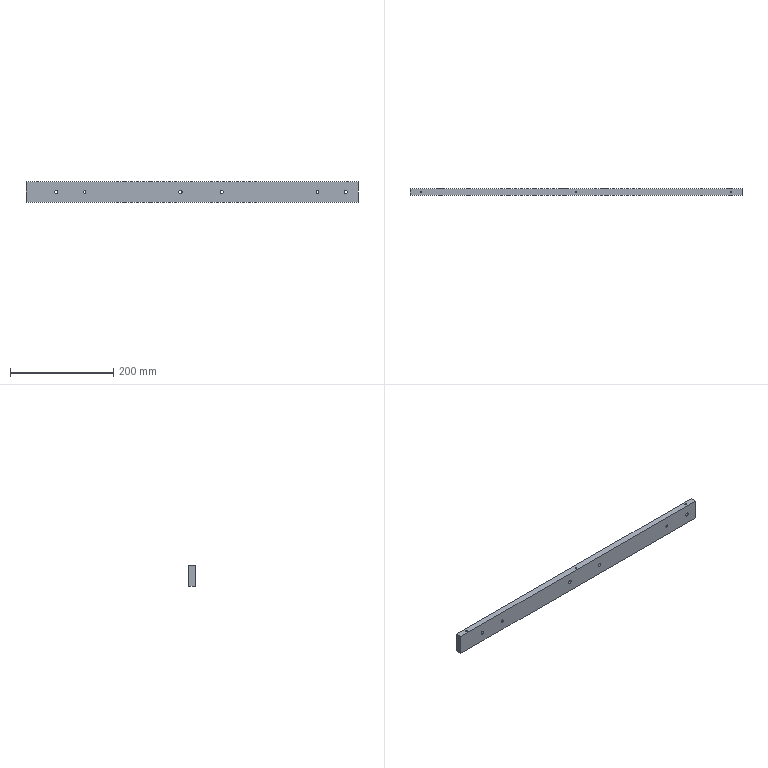Part | SolidWorks | features 3DProfileFeature 3, HoleWzd 3, Extrusion 1 | 1 solid | 42 faces | box 642 x 12 x 40 mm | volume 304076 mm3 | cylinder 26 | plane 10 | cone 6 | commonest cylinder face diameters 6.6 x8 11 x8 3.3 x6 5 x4
STEP:
#1=CARTESIAN_POINT('',(-207.5,-6.,-2.5));
#2=VERTEX_POINT('',#1);
#3=CARTESIAN_POINT('',(-207.5,-6.,2.5));
#4=VERTEX_POINT('',#3);
#5=CARTESIAN_POINT('',(-207.5,-6.,0.));
#6=DIRECTION('',(0.,1.,0.));
#7=DIRECTION('',(0.,0.,1.));
#8=AXIS2_PLACEMENT_3D('',#5,#6,#7);
#9=CIRCLE('',#8,2.5);
#10=EDGE_CURVE('',#2,#4,#9,.T.);
#11=ORIENTED_EDGE('',*,*,#10,.F.);
#12=CARTESIAN_POINT('',(-207.5,6.,-2.5));
#13=VERTEX_POINT('',#12);
#14=CARTESIAN_POINT('',(-207.5,6.,-2.5));
#15=DIRECTION('',(0.,1.,0.));
#16=VECTOR('',#15,1000.);
#17=LINE('',#14,#16);
#18=EDGE_CURVE('',#2,#13,#17,.T.);
#19=ORIENTED_EDGE('',*,*,#18,.T.);
#20=CARTESIAN_POINT('',(-207.5,6.,2.5));
#21=VERTEX_POINT('',#20);
#22=CARTESIAN_POINT('',(-207.5,6.,0.));
#23=DIRECTION('',(0.,1.,0.));
#24=DIRECTION('',(0.,0.,1.));
#25=AXIS2_PLACEMENT_3D('',#22,#23,#24);
#26=CIRCLE('',#25,2.5);
#27=EDGE_CURVE('',#13,#21,#26,.T.);
#28=ORIENTED_EDGE('',*,*,#27,.T.);
#29=CARTESIAN_POINT('',(-207.5,6.,2.5));
#30=DIRECTION('',(0.,1.,0.));
#31=VECTOR('',#30,1000.);
#32=LINE('',#29,#31);
#33=EDGE_CURVE('',#4,#21,#32,.T.);
#34=ORIENTED_EDGE('',*,*,#33,.F.);
#35=EDGE_LOOP('',(#11,#19,#28,#34));
#36=FACE_OUTER_BOUND('',#35,.T.);
#37=CARTESIAN_POINT('',(-207.5,6.,0.));
#38=DIRECTION('',(0.,1.,0.));
#39=DIRECTION('',(0.,0.,1.));
#40=AXIS2_PLACEMENT_3D('',#37,#38,#39);
#41=CYLINDRICAL_SURFACE('',#40,2.5);
#42=ADVANCED_FACE('',(#36),#41,.F.);
#43=CARTESIAN_POINT('',(242.5,-6.,-2.5));
#44=VERTEX_POINT('',#43);
#45=CARTESIAN_POINT('',(242.5,-6.,2.5));
#46=VERTEX_POINT('',#45);
#47=CARTESIAN_POINT('',(242.5,-6.,0.));
#48=DIRECTION('',(0.,1.,0.));
#49=DIRECTION('',(0.,0.,1.));
#50=AXIS2_PLACEMENT_3D('',#47,#48,#49);
#51=CIRCLE('',#50,2.5);
#52=EDGE_CURVE('',#44,#46,#51,.T.);
#53=ORIENTED_EDGE('',*,*,#52,.F.);
#54=CARTESIAN_POINT('',(242.5,6.,-2.5));
#55=VERTEX_POINT('',#54);
#56=CARTESIAN_POINT('',(242.5,6.,-2.5));
#57=DIRECTION('',(0.,1.,0.));
#58=VECTOR('',#57,1000.);
#59=LINE('',#56,#58);
#60=EDGE_CURVE('',#44,#55,#59,.T.);
#61=ORIENTED_EDGE('',*,*,#60,.T.);
#62=CARTESIAN_POINT('',(242.5,6.,2.5));
#63=VERTEX_POINT('',#62);
#64=CARTESIAN_POINT('',(242.5,6.,0.));
#65=DIRECTION('',(0.,1.,0.));
#66=DIRECTION('',(0.,0.,1.));
#67=AXIS2_PLACEMENT_3D('',#64,#65,#66);
#68=CIRCLE('',#67,2.5);
#69=EDGE_CURVE('',#55,#63,#68,.T.);
#70=ORIENTED_EDGE('',*,*,#69,.T.);
#71=CARTESIAN_POINT('',(242.5,6.,2.5));
#72=DIRECTION('',(0.,1.,0.));
#73=VECTOR('',#72,1000.);
#74=LINE('',#71,#73);
#75=EDGE_CURVE('',#46,#63,#74,.T.);
#76=ORIENTED_EDGE('',*,*,#75,.F.);
#77=EDGE_LOOP('',(#53,#61,#70,#76));
#78=FACE_OUTER_BOUND('',#77,.T.);
#79=CARTESIAN_POINT('',(242.5,6.,0.));
#80=DIRECTION('',(0.,1.,0.));
#81=DIRECTION('',(0.,0.,1.));
#82=AXIS2_PLACEMENT_3D('',#79,#80,#81);
#83=CYLINDRICAL_SURFACE('',#82,2.5);
#84=ADVANCED_FACE('',(#78),#83,.F.);
#85=CARTESIAN_POINT('',(300.,0.,8.909));
#86=VERTEX_POINT('',#85);
#87=CARTESIAN_POINT('',(301.65,0.,9.9));
#88=VERTEX_POINT('',#87);
#89=CARTESIAN_POINT('',(301.65,0.,9.9));
#90=DIRECTION('',(0.8572,0.,0.515));
#91=VECTOR('',#90,1000.);
#92=LINE('',#89,#91);
#93=EDGE_CURVE('',#86,#88,#92,.T.);
#94=ORIENTED_EDGE('',*,*,#93,.F.);
#95=CARTESIAN_POINT('',(298.35,0.,9.9));
#96=VERTEX_POINT('',#95);
#97=CARTESIAN_POINT('',(298.35,0.,9.9));
#98=DIRECTION('',(-0.8572,0.,0.515));
#99=VECTOR('',#98,1000.);
#100=LINE('',#97,#99);
#101=EDGE_CURVE('',#86,#96,#100,.T.);
#102=ORIENTED_EDGE('',*,*,#101,.T.);
#103=CARTESIAN_POINT('',(300.,0.,9.9));
#104=DIRECTION('',(0.,0.,1.));
#105=DIRECTION('',(1.,0.,0.));
#106=AXIS2_PLACEMENT_3D('',#103,#104,#105);
#107=CIRCLE('',#106,1.65);
#108=EDGE_CURVE('',#96,#88,#107,.T.);
#109=ORIENTED_EDGE('',*,*,#108,.T.);
#110=EDGE_LOOP('',(#94,#102,#109));
#111=FACE_OUTER_BOUND('',#110,.T.);
#112=CARTESIAN_POINT('',(300.,0.,9.9));
#113=DIRECTION('',(0.,0.,1.));
#114=DIRECTION('',(1.,0.,0.));
#115=AXIS2_PLACEMENT_3D('',#112,#113,#114);
#116=CONICAL_SURFACE('',#115,1.65,1.03);
#117=ADVANCED_FACE('',(#111),#116,.F.);
#118=ORIENTED_EDGE('',*,*,#108,.F.);
#119=CARTESIAN_POINT('',(298.35,0.,20.));
#120=VERTEX_POINT('',#119);
#121=CARTESIAN_POINT('',(298.35,0.,20.));
#122=DIRECTION('',(0.,0.,1.));
#123=VECTOR('',#122,1000.);
#124=LINE('',#121,#123);
#125=EDGE_CURVE('',#96,#120,#124,.T.);
#126=ORIENTED_EDGE('',*,*,#125,.T.);
#127=CARTESIAN_POINT('',(301.65,0.,20.));
#128=VERTEX_POINT('',#127);
#129=CARTESIAN_POINT('',(300.,0.,20.));
#130=DIRECTION('',(0.,0.,1.));
#131=DIRECTION('',(1.,0.,0.));
#132=AXIS2_PLACEMENT_3D('',#129,#130,#131);
#133=CIRCLE('',#132,1.65);
#134=EDGE_CURVE('',#120,#128,#133,.T.);
#135=ORIENTED_EDGE('',*,*,#134,.T.);
#136=CARTESIAN_POINT('',(301.65,0.,20.));
#137=DIRECTION('',(0.,0.,1.));
#138=VECTOR('',#137,1000.);
#139=LINE('',#136,#138);
#140=EDGE_CURVE('',#88,#128,#139,.T.);
#141=ORIENTED_EDGE('',*,*,#140,.F.);
#142=EDGE_LOOP('',(#118,#126,#135,#141));
#143=FACE_OUTER_BOUND('',#142,.T.);
#144=CARTESIAN_POINT('',(300.,0.,20.));
#145=DIRECTION('',(0.,0.,1.));
#146=DIRECTION('',(1.,0.,0.));
#147=AXIS2_PLACEMENT_3D('',#144,#145,#146);
#148=CYLINDRICAL_SURFACE('',#147,1.65);
#149=ADVANCED_FACE('',(#143),#148,.F.);
#150=CARTESIAN_POINT('',(0.,0.,8.909));
#151=VERTEX_POINT('',#150);
#152=CARTESIAN_POINT('',(1.65,0.,9.9));
#153=VERTEX_POINT('',#152);
#154=CARTESIAN_POINT('',(1.65,0.,9.9));
#155=DIRECTION('',(0.8572,0.,0.515));
#156=VECTOR('',#155,1000.);
#157=LINE('',#154,#156);
#158=EDGE_CURVE('',#151,#153,#157,.T.);
#159=ORIENTED_EDGE('',*,*,#158,.F.);
#160=CARTESIAN_POINT('',(-1.65,0.,9.9));
#161=VERTEX_POINT('',#160);
#162=CARTESIAN_POINT('',(-1.65,0.,9.9));
#163=DIRECTION('',(-0.8572,0.,0.515));
#164=VECTOR('',#163,1000.);
#165=LINE('',#162,#164);
#166=EDGE_CURVE('',#151,#161,#165,.T.);
#167=ORIENTED_EDGE('',*,*,#166,.T.);
#168=CARTESIAN_POINT('',(0.,0.,9.9));
#169=DIRECTION('',(0.,0.,1.));
#170=DIRECTION('',(1.,0.,0.));
#171=AXIS2_PLACEMENT_3D('',#168,#169,#170);
#172=CIRCLE('',#171,1.65);
#173=EDGE_CURVE('',#161,#153,#172,.T.);
#174=ORIENTED_EDGE('',*,*,#173,.T.);
#175=EDGE_LOOP('',(#159,#167,#174));
#176=FACE_OUTER_BOUND('',#175,.T.);
#177=CARTESIAN_POINT('',(0.,0.,9.9));
#178=DIRECTION('',(0.,0.,1.));
#179=DIRECTION('',(1.,0.,0.));
#180=AXIS2_PLACEMENT_3D('',#177,#178,#179);
#181=CONICAL_SURFACE('',#180,1.65,1.03);
#182=ADVANCED_FACE('',(#176),#181,.F.);
#183=ORIENTED_EDGE('',*,*,#173,.F.);
#184=CARTESIAN_POINT('',(-1.65,0.,20.));
#185=VERTEX_POINT('',#184);
#186=CARTESIAN_POINT('',(-1.65,0.,20.));
#187=DIRECTION('',(0.,0.,1.));
#188=VECTOR('',#187,1000.);
#189=LINE('',#186,#188);
#190=EDGE_CURVE('',#161,#185,#189,.T.);
#191=ORIENTED_EDGE('',*,*,#190,.T.);
#192=CARTESIAN_POINT('',(1.65,0.,20.));
#193=VERTEX_POINT('',#192);
#194=CARTESIAN_POINT('',(0.,0.,20.));
#195=DIRECTION('',(0.,0.,1.));
#196=DIRECTION('',(1.,0.,0.));
#197=AXIS2_PLACEMENT_3D('',#194,#195,#196);
#198=CIRCLE('',#197,1.65);
#199=EDGE_CURVE('',#185,#193,#198,.T.);
#200=ORIENTED_EDGE('',*,*,#199,.T.);
#201=CARTESIAN_POINT('',(1.65,0.,20.));
#202=DIRECTION('',(0.,0.,1.));
#203=VECTOR('',#202,1000.);
#204=LINE('',#201,#203);
#205=EDGE_CURVE('',#153,#193,#204,.T.);
#206=ORIENTED_EDGE('',*,*,#205,.F.);
#207=EDGE_LOOP('',(#183,#191,#200,#206));
#208=FACE_OUTER_BOUND('',#207,.T.);
#209=CARTESIAN_POINT('',(0.,0.,20.));
#210=DIRECTION('',(0.,0.,1.));
#211=DIRECTION('',(1.,0.,0.));
#212=AXIS2_PLACEMENT_3D('',#209,#210,#211);
#213=CYLINDRICAL_SURFACE('',#212,1.65);
#214=ADVANCED_FACE('',(#208),#213,.F.);
#215=CARTESIAN_POINT('',(-300.,0.,8.909));
#216=VERTEX_POINT('',#215);
#217=CARTESIAN_POINT('',(-298.35,0.,9.9));
#218=VERTEX_POINT('',#217);
#219=CARTESIAN_POINT('',(-298.35,0.,9.9));
#220=DIRECTION('',(0.8572,0.,0.515));
#221=VECTOR('',#220,1000.);
#222=LINE('',#219,#221);
#223=EDGE_CURVE('',#216,#218,#222,.T.);
#224=ORIENTED_EDGE('',*,*,#223,.F.);
#225=CARTESIAN_POINT('',(-301.65,0.,9.9));
#226=VERTEX_POINT('',#225);
#227=CARTESIAN_POINT('',(-301.65,0.,9.9));
#228=DIRECTION('',(-0.8572,0.,0.515));
#229=VECTOR('',#228,1000.);
#230=LINE('',#227,#229);
#231=EDGE_CURVE('',#216,#226,#230,.T.);
#232=ORIENTED_EDGE('',*,*,#231,.T.);
#233=CARTESIAN_POINT('',(-300.,0.,9.9));
#234=DIRECTION('',(0.,0.,1.));
#235=DIRECTION('',(1.,0.,0.));
#236=AXIS2_PLACEMENT_3D('',#233,#234,#235);
#237=CIRCLE('',#236,1.65);
#238=EDGE_CURVE('',#226,#218,#237,.T.);
#239=ORIENTED_EDGE('',*,*,#238,.T.);
#240=EDGE_LOOP('',(#224,#232,#239));
#241=FACE_OUTER_BOUND('',#240,.T.);
#242=CARTESIAN_POINT('',(-300.,0.,9.9));
#243=DIRECTION('',(0.,0.,1.));
#244=DIRECTION('',(1.,0.,0.));
#245=AXIS2_PLACEMENT_3D('',#242,#243,#244);
#246=CONICAL_SURFACE('',#245,1.65,1.03);
#247=ADVANCED_FACE('',(#241),#246,.F.);
#248=ORIENTED_EDGE('',*,*,#238,.F.);
#249=CARTESIAN_POINT('',(-301.65,0.,20.));
#250=VERTEX_POINT('',#249);
#251=CARTESIAN_POINT('',(-301.65,0.,20.));
#252=DIRECTION('',(0.,0.,1.));
#253=VECTOR('',#252,1000.);
#254=LINE('',#251,#253);
#255=EDGE_CURVE('',#226,#250,#254,.T.);
#256=ORIENTED_EDGE('',*,*,#255,.T.);
#257=CARTESIAN_POINT('',(-298.35,0.,20.));
#258=VERTEX_POINT('',#257);
#259=CARTESIAN_POINT('',(-300.,0.,20.));
#260=DIRECTION('',(0.,0.,1.));
#261=DIRECTION('',(1.,0.,0.));
#262=AXIS2_PLACEMENT_3D('',#259,#260,#261);
#263=CIRCLE('',#262,1.65);
#264=EDGE_CURVE('',#250,#258,#263,.T.);
#265=ORIENTED_EDGE('',*,*,#264,.T.);
#266=CARTESIAN_POINT('',(-298.35,0.,20.));
#267=DIRECTION('',(0.,0.,1.));
#268=VECTOR('',#267,1000.);
#269=LINE('',#266,#268);
#270=EDGE_CURVE('',#218,#258,#269,.T.);
#271=ORIENTED_EDGE('',*,*,#270,.F.);
#272=EDGE_LOOP('',(#248,#256,#265,#271));
#273=FACE_OUTER_BOUND('',#272,.T.);
#274=CARTESIAN_POINT('',(-300.,0.,20.));
#275=DIRECTION('',(0.,0.,1.));
#276=DIRECTION('',(1.,0.,0.));
#277=AXIS2_PLACEMENT_3D('',#274,#275,#276);
#278=CYLINDRICAL_SURFACE('',#277,1.65);
#279=ADVANCED_FACE('',(#273),#278,.F.);
#280=CARTESIAN_POINT('',(-262.5,-1.,-5.5));
#281=VERTEX_POINT('',#280);
#282=CARTESIAN_POINT('',(-262.5,-1.,5.5));
#283=VERTEX_POINT('',#282);
#284=CARTESIAN_POINT('',(-262.5,-1.,0.));
#285=DIRECTION('',(0.,1.,0.));
#286=DIRECTION('',(0.,0.,1.));
#287=AXIS2_PLACEMENT_3D('',#284,#285,#286);
#288=CIRCLE('',#287,5.5);
#289=EDGE_CURVE('',#281,#283,#288,.T.);
#290=ORIENTED_EDGE('',*,*,#289,.F.);
#291=CARTESIAN_POINT('',(-262.5,6.,-5.5));
#292=VERTEX_POINT('',#291);
#293=CARTESIAN_POINT('',(-262.5,6.,-5.5));
#294=DIRECTION('',(0.,1.,0.));
#295=VECTOR('',#294,1000.);
#296=LINE('',#293,#295);
#297=EDGE_CURVE('',#281,#292,#296,.T.);
#298=ORIENTED_EDGE('',*,*,#297,.T.);
#299=CARTESIAN_POINT('',(-262.5,6.,5.5));
#300=VERTEX_POINT('',#299);
#301=CARTESIAN_POINT('',(-262.5,6.,0.));
#302=DIRECTION('',(0.,1.,0.));
#303=DIRECTION('',(0.,0.,1.));
#304=AXIS2_PLACEMENT_3D('',#301,#302,#303);
#305=CIRCLE('',#304,5.5);
#306=EDGE_CURVE('',#292,#300,#305,.T.);
#307=ORIENTED_EDGE('',*,*,#306,.T.);
#308=CARTESIAN_POINT('',(-262.5,6.,5.5));
#309=DIRECTION('',(0.,1.,0.));
#310=VECTOR('',#309,1000.);
#311=LINE('',#308,#310);
#312=EDGE_CURVE('',#283,#300,#311,.T.);
#313=ORIENTED_EDGE('',*,*,#312,.F.);
#314=EDGE_LOOP('',(#290,#298,#307,#313));
#315=FACE_OUTER_BOUND('',#314,.T.);
#316=CARTESIAN_POINT('',(-262.5,6.,0.));
#317=DIRECTION('',(0.,1.,0.));
#318=DIRECTION('',(0.,0.,1.));
#319=AXIS2_PLACEMENT_3D('',#316,#317,#318);
#320=CYLINDRICAL_SURFACE('',#319,5.5);
#321=ADVANCED_FACE('',(#315),#320,.F.);
#322=CARTESIAN_POINT('',(-262.5,-6.,-3.3));
#323=VERTEX_POINT('',#322);
#324=CARTESIAN_POINT('',(-262.5,-6.,3.3));
#325=VERTEX_POINT('',#324);
#326=CARTESIAN_POINT('',(-262.5,-6.,0.));
#327=DIRECTION('',(0.,1.,0.));
#328=DIRECTION('',(0.,0.,1.));
#329=AXIS2_PLACEMENT_3D('',#326,#327,#328);
#330=CIRCLE('',#329,3.3);
#331=EDGE_CURVE('',#323,#325,#330,.T.);
#332=ORIENTED_EDGE('',*,*,#331,.F.);
#333=CARTESIAN_POINT('',(-262.5,-1.,-3.3));
#334=VERTEX_POINT('',#333);
#335=CARTESIAN_POINT('',(-262.5,6.,-3.3));
#336=DIRECTION('',(0.,1.,0.));
#337=VECTOR('',#336,1000.);
#338=LINE('',#335,#337);
#339=EDGE_CURVE('',#323,#334,#338,.T.);
#340=ORIENTED_EDGE('',*,*,#339,.T.);
#341=CARTESIAN_POINT('',(-262.5,-1.,3.3));
#342=VERTEX_POINT('',#341);
#343=CARTESIAN_POINT('',(-262.5,-1.,0.));
#344=DIRECTION('',(0.,1.,0.));
#345=DIRECTION('',(0.,0.,1.));
#346=AXIS2_PLACEMENT_3D('',#343,#344,#345);
#347=CIRCLE('',#346,3.3);
#348=EDGE_CURVE('',#334,#342,#347,.T.);
#349=ORIENTED_EDGE('',*,*,#348,.T.);
#350=CARTESIAN_POINT('',(-262.5,6.,3.3));
#351=DIRECTION('',(0.,1.,0.));
#352=VECTOR('',#351,1000.);
#353=LINE('',#350,#352);
#354=EDGE_CURVE('',#325,#342,#353,.T.);
#355=ORIENTED_EDGE('',*,*,#354,.F.);
#356=EDGE_LOOP('',(#332,#340,#349,#355));
#357=FACE_OUTER_BOUND('',#356,.T.);
#358=CARTESIAN_POINT('',(-262.5,6.,0.));
#359=DIRECTION('',(0.,1.,0.));
#360=DIRECTION('',(0.,0.,1.));
#361=AXIS2_PLACEMENT_3D('',#358,#359,#360);
#362=CYLINDRICAL_SURFACE('',#361,3.3);
#363=ADVANCED_FACE('',(#357),#362,.F.);
#364=CARTESIAN_POINT('',(-22.5,-1.,-5.5));
#365=VERTEX_POINT('',#364);
#366=CARTESIAN_POINT('',(-22.5,-1.,5.5));
#367=VERTEX_POINT('',#366);
#368=CARTESIAN_POINT('',(-22.5,-1.,0.));
#369=DIRECTION('',(0.,1.,0.));
#370=DIRECTION('',(0.,0.,1.));
#371=AXIS2_PLACEMENT_3D('',#368,#369,#370);
#372=CIRCLE('',#371,5.5);
#373=EDGE_CURVE('',#365,#367,#372,.T.);
#374=ORIENTED_EDGE('',*,*,#373,.F.);
#375=CARTESIAN_POINT('',(-22.5,6.,-5.5));
#376=VERTEX_POINT('',#375);
#377=CARTESIAN_POINT('',(-22.5,6.,-5.5));
#378=DIRECTION('',(0.,1.,0.));
#379=VECTOR('',#378,1000.);
#380=LINE('',#377,#379);
#381=EDGE_CURVE('',#365,#376,#380,.T.);
#382=ORIENTED_EDGE('',*,*,#381,.T.);
#383=CARTESIAN_POINT('',(-22.5,6.,5.5));
#384=VERTEX_POINT('',#383);
#385=CARTESIAN_POINT('',(-22.5,6.,0.));
#386=DIRECTION('',(0.,1.,0.));
#387=DIRECTION('',(0.,0.,1.));
#388=AXIS2_PLACEMENT_3D('',#385,#386,#387);
#389=CIRCLE('',#388,5.5);
#390=EDGE_CURVE('',#376,#384,#389,.T.);
#391=ORIENTED_EDGE('',*,*,#390,.T.);
#392=CARTESIAN_POINT('',(-22.5,6.,5.5));
#393=DIRECTION('',(0.,1.,0.));
#394=VECTOR('',#393,1000.);
#395=LINE('',#392,#394);
#396=EDGE_CURVE('',#367,#384,#395,.T.);
#397=ORIENTED_EDGE('',*,*,#396,.F.);
#398=EDGE_LOOP('',(#374,#382,#391,#397));
#399=FACE_OUTER_BOUND('',#398,.T.);
#400=CARTESIAN_POINT('',(-22.5,6.,0.));
#401=DIRECTION('',(0.,1.,0.));
#402=DIRECTION('',(0.,0.,1.));
#403=AXIS2_PLACEMENT_3D('',#400,#401,#402);
#404=CYLINDRICAL_SURFACE('',#403,5.5);
#405=ADVANCED_FACE('',(#399),#404,.F.);
#406=CARTESIAN_POINT('',(-22.5,-6.,-3.3));
#407=VERTEX_POINT('',#406);
#408=CARTESIAN_POINT('',(-22.5,-6.,3.3));
#409=VERTEX_POINT('',#408);
#410=CARTESIAN_POINT('',(-22.5,-6.,0.));
#411=DIRECTION('',(0.,1.,0.));
#412=DIRECTION('',(0.,0.,1.));
#413=AXIS2_PLACEMENT_3D('',#410,#411,#412);
#414=CIRCLE('',#413,3.3);
#415=EDGE_CURVE('',#407,#409,#414,.T.);
#416=ORIENTED_EDGE('',*,*,#415,.F.);
#417=CARTESIAN_POINT('',(-22.5,-1.,-3.3));
#418=VERTEX_POINT('',#417);
#419=CARTESIAN_POINT('',(-22.5,6.,-3.3));
#420=DIRECTION('',(0.,1.,0.));
#421=VECTOR('',#420,1000.);
#422=LINE('',#419,#421);
#423=EDGE_CURVE('',#407,#418,#422,.T.);
#424=ORIENTED_EDGE('',*,*,#423,.T.);
#425=CARTESIAN_POINT('',(-22.5,-1.,3.3));
#426=VERTEX_POINT('',#425);
#427=CARTESIAN_POINT('',(-22.5,-1.,0.));
#428=DIRECTION('',(0.,1.,0.));
#429=DIRECTION('',(0.,0.,1.));
#430=AXIS2_PLACEMENT_3D('',#427,#428,#429);
#431=CIRCLE('',#430,3.3);
#432=EDGE_CURVE('',#418,#426,#431,.T.);
#433=ORIENTED_EDGE('',*,*,#432,.T.);
#434=CARTESIAN_POINT('',(-22.5,6.,3.3));
#435=DIRECTION('',(0.,1.,0.));
#436=VECTOR('',#435,1000.);
#437=LINE('',#434,#436);
#438=EDGE_CURVE('',#409,#426,#437,.T.);
#439=ORIENTED_EDGE('',*,*,#438,.F.);
#440=EDGE_LOOP('',(#416,#424,#433,#439));
#441=FACE_OUTER_BOUND('',#440,.T.);
#442=CARTESIAN_POINT('',(-22.5,6.,0.));
#443=DIRECTION('',(0.,1.,0.));
#444=DIRECTION('',(0.,0.,1.));
#445=AXIS2_PLACEMENT_3D('',#442,#443,#444);
#446=CYLINDRICAL_SURFACE('',#445,3.3);
#447=ADVANCED_FACE('',(#441),#446,.F.);
#448=CARTESIAN_POINT('',(57.5,-1.,-5.5));
#449=VERTEX_POINT('',#448);
#450=CARTESIAN_POINT('',(57.5,-1.,5.5));
#451=VERTEX_POINT('',#450);
#452=CARTESIAN_POINT('',(57.5,-1.,0.));
#453=DIRECTION('',(0.,1.,0.));
#454=DIRECTION('',(0.,0.,1.));
#455=AXIS2_PLACEMENT_3D('',#452,#453,#454);
#456=CIRCLE('',#455,5.5);
#457=EDGE_CURVE('',#449,#451,#456,.T.);
#458=ORIENTED_EDGE('',*,*,#457,.F.);
#459=CARTESIAN_POINT('',(57.5,6.,-5.5));
#460=VERTEX_POINT('',#459);
#461=CARTESIAN_POINT('',(57.5,6.,-5.5));
#462=DIRECTION('',(0.,1.,0.));
#463=VECTOR('',#462,1000.);
#464=LINE('',#461,#463);
#465=EDGE_CURVE('',#449,#460,#464,.T.);
#466=ORIENTED_EDGE('',*,*,#465,.T.);
#467=CARTESIAN_POINT('',(57.5,6.,5.5));
#468=VERTEX_POINT('',#467);
#469=CARTESIAN_POINT('',(57.5,6.,0.));
#470=DIRECTION('',(0.,1.,0.));
#471=DIRECTION('',(0.,0.,1.));
#472=AXIS2_PLACEMENT_3D('',#469,#470,#471);
#473=CIRCLE('',#472,5.5);
#474=EDGE_CURVE('',#460,#468,#473,.T.);
#475=ORIENTED_EDGE('',*,*,#474,.T.);
#476=CARTESIAN_POINT('',(57.5,6.,5.5));
#477=DIRECTION('',(0.,1.,0.));
#478=VECTOR('',#477,1000.);
#479=LINE('',#476,#478);
#480=EDGE_CURVE('',#451,#468,#479,.T.);
#481=ORIENTED_EDGE('',*,*,#480,.F.);
#482=EDGE_LOOP('',(#458,#466,#475,#481));
#483=FACE_OUTER_BOUND('',#482,.T.);
#484=CARTESIAN_POINT('',(57.5,6.,0.));
#485=DIRECTION('',(0.,1.,0.));
#486=DIRECTION('',(0.,0.,1.));
#487=AXIS2_PLACEMENT_3D('',#484,#485,#486);
#488=CYLINDRICAL_SURFACE('',#487,5.5);
#489=ADVANCED_FACE('',(#483),#488,.F.);
#490=CARTESIAN_POINT('',(57.5,-6.,-3.3));
#491=VERTEX_POINT('',#490);
#492=CARTESIAN_POINT('',(57.5,-6.,3.3));
#493=VERTEX_POINT('',#492);
#494=CARTESIAN_POINT('',(57.5,-6.,0.));
#495=DIRECTION('',(0.,1.,0.));
#496=DIRECTION('',(0.,0.,1.));
#497=AXIS2_PLACEMENT_3D('',#494,#495,#496);
#498=CIRCLE('',#497,3.3);
#499=EDGE_CURVE('',#491,#493,#498,.T.);
#500=ORIENTED_EDGE('',*,*,#499,.F.);
#501=CARTESIAN_POINT('',(57.5,-1.,-3.3));
#502=VERTEX_POINT('',#501);
#503=CARTESIAN_POINT('',(57.5,6.,-3.3));
#504=DIRECTION('',(0.,1.,0.));
#505=VECTOR('',#504,1000.);
#506=LINE('',#503,#505);
#507=EDGE_CURVE('',#491,#502,#506,.T.);
#508=ORIENTED_EDGE('',*,*,#507,.T.);
#509=CARTESIAN_POINT('',(57.5,-1.,3.3));
#510=VERTEX_POINT('',#509);
#511=CARTESIAN_POINT('',(57.5,-1.,0.));
#512=DIRECTION('',(0.,1.,0.));
#513=DIRECTION('',(0.,0.,1.));
#514=AXIS2_PLACEMENT_3D('',#511,#512,#513);
#515=CIRCLE('',#514,3.3);
#516=EDGE_CURVE('',#502,#510,#515,.T.);
#517=ORIENTED_EDGE('',*,*,#516,.T.);
#518=CARTESIAN_POINT('',(57.5,6.,3.3));
#519=DIRECTION('',(0.,1.,0.));
#520=VECTOR('',#519,1000.);
#521=LINE('',#518,#520);
#522=EDGE_CURVE('',#493,#510,#521,.T.);
#523=ORIENTED_EDGE('',*,*,#522,.F.);
#524=EDGE_LOOP('',(#500,#508,#517,#523));
#525=FACE_OUTER_BOUND('',#524,.T.);
#526=CARTESIAN_POINT('',(57.5,6.,0.));
#527=DIRECTION('',(0.,1.,0.));
#528=DIRECTION('',(0.,0.,1.));
#529=AXIS2_PLACEMENT_3D('',#526,#527,#528);
#530=CYLINDRICAL_SURFACE('',#529,3.3);
#531=ADVANCED_FACE('',(#525),#530,.F.);
#532=CARTESIAN_POINT('',(297.5,-1.,-5.5));
#533=VERTEX_POINT('',#532);
#534=CARTESIAN_POINT('',(297.5,-1.,5.5));
#535=VERTEX_POINT('',#534);
#536=CARTESIAN_POINT('',(297.5,-1.,0.));
#537=DIRECTION('',(0.,1.,0.));
#538=DIRECTION('',(0.,0.,1.));
#539=AXIS2_PLACEMENT_3D('',#536,#537,#538);
#540=CIRCLE('',#539,5.5);
#541=EDGE_CURVE('',#533,#535,#540,.T.);
#542=ORIENTED_EDGE('',*,*,#541,.F.);
#543=CARTESIAN_POINT('',(297.5,6.,-5.5));
#544=VERTEX_POINT('',#543);
#545=CARTESIAN_POINT('',(297.5,6.,-5.5));
#546=DIRECTION('',(0.,1.,0.));
#547=VECTOR('',#546,1000.);
#548=LINE('',#545,#547);
#549=EDGE_CURVE('',#533,#544,#548,.T.);
#550=ORIENTED_EDGE('',*,*,#549,.T.);
#551=CARTESIAN_POINT('',(297.5,6.,5.5));
#552=VERTEX_POINT('',#551);
#553=CARTESIAN_POINT('',(297.5,6.,0.));
#554=DIRECTION('',(0.,1.,0.));
#555=DIRECTION('',(0.,0.,1.));
#556=AXIS2_PLACEMENT_3D('',#553,#554,#555);
#557=CIRCLE('',#556,5.5);
#558=EDGE_CURVE('',#544,#552,#557,.T.);
#559=ORIENTED_EDGE('',*,*,#558,.T.);
#560=CARTESIAN_POINT('',(297.5,6.,5.5));
#561=DIRECTION('',(0.,1.,0.));
#562=VECTOR('',#561,1000.);
#563=LINE('',#560,#562);
#564=EDGE_CURVE('',#535,#552,#563,.T.);
#565=ORIENTED_EDGE('',*,*,#564,.F.);
#566=EDGE_LOOP('',(#542,#550,#559,#565));
#567=FACE_OUTER_BOUND('',#566,.T.);
#568=CARTESIAN_POINT('',(297.5,6.,0.));
#569=DIRECTION('',(0.,1.,0.));
#570=DIRECTION('',(0.,0.,1.));
#571=AXIS2_PLACEMENT_3D('',#568,#569,#570);
#572=CYLINDRICAL_SURFACE('',#571,5.5);
#573=ADVANCED_FACE('',(#567),#572,.F.);
#574=CARTESIAN_POINT('',(297.5,-6.,-3.3));
#575=VERTEX_POINT('',#574);
#576=CARTESIAN_POINT('',(297.5,-6.,3.3));
#577=VERTEX_POINT('',#576);
#578=CARTESIAN_POINT('',(297.5,-6.,0.));
#579=DIRECTION('',(0.,1.,0.));
#580=DIRECTION('',(0.,0.,1.));
#581=AXIS2_PLACEMENT_3D('',#578,#579,#580);
#582=CIRCLE('',#581,3.3);
#583=EDGE_CURVE('',#575,#577,#582,.T.);
#584=ORIENTED_EDGE('',*,*,#583,.F.);
#585=CARTESIAN_POINT('',(297.5,-1.,-3.3));
#586=VERTEX_POINT('',#585);
#587=CARTESIAN_POINT('',(297.5,6.,-3.3));
#588=DIRECTION('',(0.,1.,0.));
#589=VECTOR('',#588,1000.);
#590=LINE('',#587,#589);
#591=EDGE_CURVE('',#575,#586,#590,.T.);
#592=ORIENTED_EDGE('',*,*,#591,.T.);
#593=CARTESIAN_POINT('',(297.5,-1.,3.3));
#594=VERTEX_POINT('',#593);
#595=CARTESIAN_POINT('',(297.5,-1.,0.));
#596=DIRECTION('',(0.,1.,0.));
#597=DIRECTION('',(0.,0.,1.));
#598=AXIS2_PLACEMENT_3D('',#595,#596,#597);
#599=CIRCLE('',#598,3.3);
#600=EDGE_CURVE('',#586,#594,#599,.T.);
#601=ORIENTED_EDGE('',*,*,#600,.T.);
#602=CARTESIAN_POINT('',(297.5,6.,3.3));
#603=DIRECTION('',(0.,1.,0.));
#604=VECTOR('',#603,1000.);
#605=LINE('',#602,#604);
#606=EDGE_CURVE('',#577,#594,#605,.T.);
#607=ORIENTED_EDGE('',*,*,#606,.F.);
#608=EDGE_LOOP('',(#584,#592,#601,#607));
#609=FACE_OUTER_BOUND('',#608,.T.);
#610=CARTESIAN_POINT('',(297.5,6.,0.));
#611=DIRECTION('',(0.,1.,0.));
#612=DIRECTION('',(0.,0.,1.));
#613=AXIS2_PLACEMENT_3D('',#610,#611,#612);
#614=CYLINDRICAL_SURFACE('',#613,3.3);
#615=ADVANCED_FACE('',(#609),#614,.F.);
#616=CARTESIAN_POINT('',(-321.,-6.,-20.));
#617=VERTEX_POINT('',#616);
#618=CARTESIAN_POINT('',(-321.,-6.,20.));
#619=VERTEX_POINT('',#618);
#620=CARTESIAN_POINT('',(-321.,-6.,-20.));
#621=DIRECTION('',(0.,0.,1.));
#622=VECTOR('',#621,1000.);
#623=LINE('',#620,#622);
#624=EDGE_CURVE('',#617,#619,#623,.T.);
#625=ORIENTED_EDGE('',*,*,#624,.T.);
#626=CARTESIAN_POINT('',(-321.,6.,20.));
#627=VERTEX_POINT('',#626);
#628=CARTESIAN_POINT('',(-321.,6.,20.));
#629=DIRECTION('',(0.,-1.,0.));
#630=VECTOR('',#629,1000.);
#631=LINE('',#628,#630);
#632=EDGE_CURVE('',#627,#619,#631,.T.);
#633=ORIENTED_EDGE('',*,*,#632,.F.);
#634=CARTESIAN_POINT('',(-321.,6.,-20.));
#635=VERTEX_POINT('',#634);
#636=CARTESIAN_POINT('',(-321.,6.,-20.));
#637=DIRECTION('',(0.,0.,1.));
#638=VECTOR('',#637,1000.);
#639=LINE('',#636,#638);
#640=EDGE_CURVE('',#635,#627,#639,.T.);
#641=ORIENTED_EDGE('',*,*,#640,.F.);
#642=CARTESIAN_POINT('',(-321.,6.,-20.));
#643=DIRECTION('',(0.,-1.,0.));
#644=VECTOR('',#643,1000.);
#645=LINE('',#642,#644);
#646=EDGE_CURVE('',#635,#617,#645,.T.);
#647=ORIENTED_EDGE('',*,*,#646,.T.);
#648=EDGE_LOOP('',(#625,#633,#641,#647));
#649=FACE_OUTER_BOUND('',#648,.T.);
#650=CARTESIAN_POINT('',(-321.,6.,-20.));
#651=DIRECTION('',(1.,0.,0.));
#652=DIRECTION('',(0.,0.,-1.));
#653=AXIS2_PLACEMENT_3D('',#650,#651,#652);
#654=PLANE('',#653);
#655=ADVANCED_FACE('',(#649),#654,.F.);
#656=CARTESIAN_POINT('',(300.,0.,20.));
#657=DIRECTION('',(0.,0.,1.));
#658=DIRECTION('',(1.,0.,0.));
#659=AXIS2_PLACEMENT_3D('',#656,#657,#658);
#660=CIRCLE('',#659,1.65);
#661=EDGE_CURVE('',#128,#120,#660,.T.);
#662=ORIENTED_EDGE('',*,*,#661,.F.);
#663=ORIENTED_EDGE('',*,*,#134,.F.);
#664=EDGE_LOOP('',(#662,#663));
#665=FACE_BOUND('',#664,.T.);
#666=CARTESIAN_POINT('',(0.,0.,20.));
#667=DIRECTION('',(0.,0.,1.));
#668=DIRECTION('',(1.,0.,0.));
#669=AXIS2_PLACEMENT_3D('',#666,#667,#668);
#670=CIRCLE('',#669,1.65);
#671=EDGE_CURVE('',#193,#185,#670,.T.);
#672=ORIENTED_EDGE('',*,*,#671,.F.);
#673=ORIENTED_EDGE('',*,*,#199,.F.);
#674=EDGE_LOOP('',(#672,#673));
#675=FACE_BOUND('',#674,.T.);
#676=CARTESIAN_POINT('',(-300.,0.,20.));
#677=DIRECTION('',(0.,0.,1.));
#678=DIRECTION('',(1.,0.,0.));
#679=AXIS2_PLACEMENT_3D('',#676,#677,#678);
#680=CIRCLE('',#679,1.65);
#681=EDGE_CURVE('',#258,#250,#680,.T.);
#682=ORIENTED_EDGE('',*,*,#681,.F.);
#683=ORIENTED_EDGE('',*,*,#264,.F.);
#684=EDGE_LOOP('',(#682,#683));
#685=FACE_BOUND('',#684,.T.);
#686=CARTESIAN_POINT('',(321.,-6.,20.));
#687=VERTEX_POINT('',#686);
#688=CARTESIAN_POINT('',(-321.,-6.,20.));
#689=DIRECTION('',(1.,0.,0.));
#690=VECTOR('',#689,1000.);
#691=LINE('',#688,#690);
#692=EDGE_CURVE('',#619,#687,#691,.T.);
#693=ORIENTED_EDGE('',*,*,#692,.T.);
#694=CARTESIAN_POINT('',(321.,6.,20.));
#695=VERTEX_POINT('',#694);
#696=CARTESIAN_POINT('',(321.,6.,20.));
#697=DIRECTION('',(0.,-1.,0.));
#698=VECTOR('',#697,1000.);
#699=LINE('',#696,#698);
#700=EDGE_CURVE('',#695,#687,#699,.T.);
#701=ORIENTED_EDGE('',*,*,#700,.F.);
#702=CARTESIAN_POINT('',(-321.,6.,20.));
#703=DIRECTION('',(1.,0.,0.));
#704=VECTOR('',#703,1000.);
#705=LINE('',#702,#704);
#706=EDGE_CURVE('',#627,#695,#705,.T.);
#707=ORIENTED_EDGE('',*,*,#706,.F.);
#708=ORIENTED_EDGE('',*,*,#632,.T.);
#709=EDGE_LOOP('',(#693,#701,#707,#708));
#710=FACE_OUTER_BOUND('',#709,.T.);
#711=CARTESIAN_POINT('',(-321.,6.,20.));
#712=DIRECTION('',(0.,0.,-1.));
#713=DIRECTION('',(-1.,0.,0.));
#714=AXIS2_PLACEMENT_3D('',#711,#712,#713);
#715=PLANE('',#714);
#716=ADVANCED_FACE('',(#665,#675,#685,#710),#715,.F.);
#717=CARTESIAN_POINT('',(321.,-6.,-20.));
#718=VERTEX_POINT('',#717);
#719=CARTESIAN_POINT('',(321.,-6.,-20.));
#720=DIRECTION('',(0.,0.,-1.));
#721=VECTOR('',#720,1000.);
#722=LINE('',#719,#721);
#723=EDGE_CURVE('',#687,#718,#722,.T.);
#724=ORIENTED_EDGE('',*,*,#723,.T.);
#725=CARTESIAN_POINT('',(321.,6.,-20.));
#726=VERTEX_POINT('',#725);
#727=CARTESIAN_POINT('',(321.,6.,-20.));
#728=DIRECTION('',(0.,-1.,0.));
#729=VECTOR('',#728,1000.);
#730=LINE('',#727,#729);
#731=EDGE_CURVE('',#726,#718,#730,.T.);
#732=ORIENTED_EDGE('',*,*,#731,.F.);
#733=CARTESIAN_POINT('',(321.,6.,-20.));
#734=DIRECTION('',(0.,0.,-1.));
#735=VECTOR('',#734,1000.);
#736=LINE('',#733,#735);
#737=EDGE_CURVE('',#695,#726,#736,.T.);
#738=ORIENTED_EDGE('',*,*,#737,.F.);
#739=ORIENTED_EDGE('',*,*,#700,.T.);
#740=EDGE_LOOP('',(#724,#732,#738,#739));
#741=FACE_OUTER_BOUND('',#740,.T.);
#742=CARTESIAN_POINT('',(321.,6.,-20.));
#743=DIRECTION('',(-1.,0.,0.));
#744=DIRECTION('',(0.,0.,1.));
#745=AXIS2_PLACEMENT_3D('',#742,#743,#744);
#746=PLANE('',#745);
#747=ADVANCED_FACE('',(#741),#746,.F.);
#748=CARTESIAN_POINT('',(-321.,-6.,-20.));
#749=DIRECTION('',(-1.,0.,0.));
#750=VECTOR('',#749,1000.);
#751=LINE('',#748,#750);
#752=EDGE_CURVE('',#718,#617,#751,.T.);
#753=ORIENTED_EDGE('',*,*,#752,.T.);
#754=ORIENTED_EDGE('',*,*,#646,.F.);
#755=CARTESIAN_POINT('',(-321.,6.,-20.));
#756=DIRECTION('',(-1.,0.,0.));
#757=VECTOR('',#756,1000.);
#758=LINE('',#755,#757);
#759=EDGE_CURVE('',#726,#635,#758,.T.);
#760=ORIENTED_EDGE('',*,*,#759,.F.);
#761=ORIENTED_EDGE('',*,*,#731,.T.);
#762=EDGE_LOOP('',(#753,#754,#760,#761));
#763=FACE_OUTER_BOUND('',#762,.T.);
#764=CARTESIAN_POINT('',(-321.,6.,-20.));
#765=DIRECTION('',(0.,0.,1.));
#766=DIRECTION('',(1.,0.,0.));
#767=AXIS2_PLACEMENT_3D('',#764,#765,#766);
#768=PLANE('',#767);
#769=ADVANCED_FACE('',(#763),#768,.F.);
#770=CARTESIAN_POINT('',(-207.5,6.,0.));
#771=DIRECTION('',(0.,1.,0.));
#772=DIRECTION('',(0.,0.,1.));
#773=AXIS2_PLACEMENT_3D('',#770,#771,#772);
#774=CIRCLE('',#773,2.5);
#775=EDGE_CURVE('',#21,#13,#774,.T.);
#776=ORIENTED_EDGE('',*,*,#775,.F.);
#777=ORIENTED_EDGE('',*,*,#27,.F.);
#778=EDGE_LOOP('',(#776,#777));
#779=FACE_BOUND('',#778,.T.);
#780=CARTESIAN_POINT('',(242.5,6.,0.));
#781=DIRECTION('',(0.,1.,0.));
#782=DIRECTION('',(0.,0.,1.));
#783=AXIS2_PLACEMENT_3D('',#780,#781,#782);
#784=CIRCLE('',#783,2.5);
#785=EDGE_CURVE('',#63,#55,#784,.T.);
#786=ORIENTED_EDGE('',*,*,#785,.F.);
#787=ORIENTED_EDGE('',*,*,#69,.F.);
#788=EDGE_LOOP('',(#786,#787));
#789=FACE_BOUND('',#788,.T.);
#790=CARTESIAN_POINT('',(-262.5,6.,0.));
#791=DIRECTION('',(0.,1.,0.));
#792=DIRECTION('',(0.,0.,1.));
#793=AXIS2_PLACEMENT_3D('',#790,#791,#792);
#794=CIRCLE('',#793,5.5);
#795=EDGE_CURVE('',#300,#292,#794,.T.);
#796=ORIENTED_EDGE('',*,*,#795,.F.);
#797=ORIENTED_EDGE('',*,*,#306,.F.);
#798=EDGE_LOOP('',(#796,#797));
#799=FACE_BOUND('',#798,.T.);
#800=CARTESIAN_POINT('',(-22.5,6.,0.));
#801=DIRECTION('',(0.,1.,0.));
#802=DIRECTION('',(0.,0.,1.));
#803=AXIS2_PLACEMENT_3D('',#800,#801,#802);
#804=CIRCLE('',#803,5.5);
#805=EDGE_CURVE('',#384,#376,#804,.T.);
#806=ORIENTED_EDGE('',*,*,#805,.F.);
#807=ORIENTED_EDGE('',*,*,#390,.F.);
#808=EDGE_LOOP('',(#806,#807));
#809=FACE_BOUND('',#808,.T.);
#810=CARTESIAN_POINT('',(57.5,6.,0.));
#811=DIRECTION('',(0.,1.,0.));
#812=DIRECTION('',(0.,0.,1.));
#813=AXIS2_PLACEMENT_3D('',#810,#811,#812);
#814=CIRCLE('',#813,5.5);
#815=EDGE_CURVE('',#468,#460,#814,.T.);
#816=ORIENTED_EDGE('',*,*,#815,.F.);
#817=ORIENTED_EDGE('',*,*,#474,.F.);
#818=EDGE_LOOP('',(#816,#817));
#819=FACE_BOUND('',#818,.T.);
#820=CARTESIAN_POINT('',(297.5,6.,0.));
#821=DIRECTION('',(0.,1.,0.));
#822=DIRECTION('',(0.,0.,1.));
#823=AXIS2_PLACEMENT_3D('',#820,#821,#822);
#824=CIRCLE('',#823,5.5);
#825=EDGE_CURVE('',#552,#544,#824,.T.);
#826=ORIENTED_EDGE('',*,*,#825,.F.);
#827=ORIENTED_EDGE('',*,*,#558,.F.);
#828=EDGE_LOOP('',(#826,#827));
#829=FACE_BOUND('',#828,.T.);
#830=ORIENTED_EDGE('',*,*,#640,.T.);
#831=ORIENTED_EDGE('',*,*,#706,.T.);
#832=ORIENTED_EDGE('',*,*,#737,.T.);
#833=ORIENTED_EDGE('',*,*,#759,.T.);
#834=EDGE_LOOP('',(#830,#831,#832,#833));
#835=FACE_OUTER_BOUND('',#834,.T.);
#836=CARTESIAN_POINT('',(-321.,6.,20.));
#837=DIRECTION('',(0.,1.,0.));
#838=DIRECTION('',(0.,0.,1.));
#839=AXIS2_PLACEMENT_3D('',#836,#837,#838);
#840=PLANE('',#839);
#841=ADVANCED_FACE('',(#779,#789,#799,#809,#819,#829,#835),#840,.T.);
#842=CARTESIAN_POINT('',(-207.5,-6.,0.));
#843=DIRECTION('',(0.,1.,0.));
#844=DIRECTION('',(0.,0.,1.));
#845=AXIS2_PLACEMENT_3D('',#842,#843,#844);
#846=CIRCLE('',#845,2.5);
#847=EDGE_CURVE('',#4,#2,#846,.T.);
#848=ORIENTED_EDGE('',*,*,#847,.T.);
#849=ORIENTED_EDGE('',*,*,#10,.T.);
#850=EDGE_LOOP('',(#848,#849));
#851=FACE_BOUND('',#850,.T.);
#852=CARTESIAN_POINT('',(242.5,-6.,0.));
#853=DIRECTION('',(0.,1.,0.));
#854=DIRECTION('',(0.,0.,1.));
#855=AXIS2_PLACEMENT_3D('',#852,#853,#854);
#856=CIRCLE('',#855,2.5);
#857=EDGE_CURVE('',#46,#44,#856,.T.);
#858=ORIENTED_EDGE('',*,*,#857,.T.);
#859=ORIENTED_EDGE('',*,*,#52,.T.);
#860=EDGE_LOOP('',(#858,#859));
#861=FACE_BOUND('',#860,.T.);
#862=CARTESIAN_POINT('',(-262.5,-6.,0.));
#863=DIRECTION('',(0.,1.,0.));
#864=DIRECTION('',(0.,0.,1.));
#865=AXIS2_PLACEMENT_3D('',#862,#863,#864);
#866=CIRCLE('',#865,3.3);
#867=EDGE_CURVE('',#325,#323,#866,.T.);
#868=ORIENTED_EDGE('',*,*,#867,.T.);
#869=ORIENTED_EDGE('',*,*,#331,.T.);
#870=EDGE_LOOP('',(#868,#869));
#871=FACE_BOUND('',#870,.T.);
#872=CARTESIAN_POINT('',(-22.5,-6.,0.));
#873=DIRECTION('',(0.,1.,0.));
#874=DIRECTION('',(0.,0.,1.));
#875=AXIS2_PLACEMENT_3D('',#872,#873,#874);
#876=CIRCLE('',#875,3.3);
#877=EDGE_CURVE('',#409,#407,#876,.T.);
#878=ORIENTED_EDGE('',*,*,#877,.T.);
#879=ORIENTED_EDGE('',*,*,#415,.T.);
#880=EDGE_LOOP('',(#878,#879));
#881=FACE_BOUND('',#880,.T.);
#882=CARTESIAN_POINT('',(57.5,-6.,0.));
#883=DIRECTION('',(0.,1.,0.));
#884=DIRECTION('',(0.,0.,1.));
#885=AXIS2_PLACEMENT_3D('',#882,#883,#884);
#886=CIRCLE('',#885,3.3);
#887=EDGE_CURVE('',#493,#491,#886,.T.);
#888=ORIENTED_EDGE('',*,*,#887,.T.);
#889=ORIENTED_EDGE('',*,*,#499,.T.);
#890=EDGE_LOOP('',(#888,#889));
#891=FACE_BOUND('',#890,.T.);
#892=CARTESIAN_POINT('',(297.5,-6.,0.));
#893=DIRECTION('',(0.,1.,0.));
#894=DIRECTION('',(0.,0.,1.));
#895=AXIS2_PLACEMENT_3D('',#892,#893,#894);
#896=CIRCLE('',#895,3.3);
#897=EDGE_CURVE('',#577,#575,#896,.T.);
#898=ORIENTED_EDGE('',*,*,#897,.T.);
#899=ORIENTED_EDGE('',*,*,#583,.T.);
#900=EDGE_LOOP('',(#898,#899));
#901=FACE_BOUND('',#900,.T.);
#902=ORIENTED_EDGE('',*,*,#624,.F.);
#903=ORIENTED_EDGE('',*,*,#752,.F.);
#904=ORIENTED_EDGE('',*,*,#723,.F.);
#905=ORIENTED_EDGE('',*,*,#692,.F.);
#906=EDGE_LOOP('',(#902,#903,#904,#905));
#907=FACE_OUTER_BOUND('',#906,.T.);
#908=CARTESIAN_POINT('',(-321.,-6.,20.));
#909=DIRECTION('',(0.,1.,0.));
#910=DIRECTION('',(0.,0.,1.));
#911=AXIS2_PLACEMENT_3D('',#908,#909,#910);
#912=PLANE('',#911);
#913=ADVANCED_FACE('',(#851,#861,#871,#881,#891,#901,#907),#912,.F.);
#914=ORIENTED_EDGE('',*,*,#591,.F.);
#915=ORIENTED_EDGE('',*,*,#897,.F.);
#916=ORIENTED_EDGE('',*,*,#606,.T.);
#917=CARTESIAN_POINT('',(297.5,-1.,0.));
#918=DIRECTION('',(0.,1.,0.));
#919=DIRECTION('',(0.,0.,1.));
#920=AXIS2_PLACEMENT_3D('',#917,#918,#919);
#921=CIRCLE('',#920,3.3);
#922=EDGE_CURVE('',#594,#586,#921,.T.);
#923=ORIENTED_EDGE('',*,*,#922,.T.);
#924=EDGE_LOOP('',(#914,#915,#916,#923));
#925=FACE_OUTER_BOUND('',#924,.T.);
#926=CARTESIAN_POINT('',(297.5,6.,0.));
#927=DIRECTION('',(0.,1.,0.));
#928=DIRECTION('',(0.,0.,1.));
#929=AXIS2_PLACEMENT_3D('',#926,#927,#928);
#930=CYLINDRICAL_SURFACE('',#929,3.3);
#931=ADVANCED_FACE('',(#925),#930,.F.);
#932=ORIENTED_EDGE('',*,*,#922,.F.);
#933=ORIENTED_EDGE('',*,*,#600,.F.);
#934=EDGE_LOOP('',(#932,#933));
#935=FACE_BOUND('',#934,.T.);
#936=CARTESIAN_POINT('',(297.5,-1.,0.));
#937=DIRECTION('',(0.,1.,0.));
#938=DIRECTION('',(0.,0.,1.));
#939=AXIS2_PLACEMENT_3D('',#936,#937,#938);
#940=CIRCLE('',#939,5.5);
#941=EDGE_CURVE('',#535,#533,#940,.T.);
#942=ORIENTED_EDGE('',*,*,#941,.T.);
#943=ORIENTED_EDGE('',*,*,#541,.T.);
#944=EDGE_LOOP('',(#942,#943));
#945=FACE_OUTER_BOUND('',#944,.T.);
#946=CARTESIAN_POINT('',(300.8,-1.,0.));
#947=DIRECTION('',(0.,-1.,0.));
#948=DIRECTION('',(0.,0.,-1.));
#949=AXIS2_PLACEMENT_3D('',#946,#947,#948);
#950=PLANE('',#949);
#951=ADVANCED_FACE('',(#935,#945),#950,.F.);
#952=ORIENTED_EDGE('',*,*,#549,.F.);
#953=ORIENTED_EDGE('',*,*,#941,.F.);
#954=ORIENTED_EDGE('',*,*,#564,.T.);
#955=ORIENTED_EDGE('',*,*,#825,.T.);
#956=EDGE_LOOP('',(#952,#953,#954,#955));
#957=FACE_OUTER_BOUND('',#956,.T.);
#958=CARTESIAN_POINT('',(297.5,6.,0.));
#959=DIRECTION('',(0.,1.,0.));
#960=DIRECTION('',(0.,0.,1.));
#961=AXIS2_PLACEMENT_3D('',#958,#959,#960);
#962=CYLINDRICAL_SURFACE('',#961,5.5);
#963=ADVANCED_FACE('',(#957),#962,.F.);
#964=ORIENTED_EDGE('',*,*,#507,.F.);
#965=ORIENTED_EDGE('',*,*,#887,.F.);
#966=ORIENTED_EDGE('',*,*,#522,.T.);
#967=CARTESIAN_POINT('',(57.5,-1.,0.));
#968=DIRECTION('',(0.,1.,0.));
#969=DIRECTION('',(0.,0.,1.));
#970=AXIS2_PLACEMENT_3D('',#967,#968,#969);
#971=CIRCLE('',#970,3.3);
#972=EDGE_CURVE('',#510,#502,#971,.T.);
#973=ORIENTED_EDGE('',*,*,#972,.T.);
#974=EDGE_LOOP('',(#964,#965,#966,#973));
#975=FACE_OUTER_BOUND('',#974,.T.);
#976=CARTESIAN_POINT('',(57.5,6.,0.));
#977=DIRECTION('',(0.,1.,0.));
#978=DIRECTION('',(0.,0.,1.));
#979=AXIS2_PLACEMENT_3D('',#976,#977,#978);
#980=CYLINDRICAL_SURFACE('',#979,3.3);
#981=ADVANCED_FACE('',(#975),#980,.F.);
#982=ORIENTED_EDGE('',*,*,#972,.F.);
#983=ORIENTED_EDGE('',*,*,#516,.F.);
#984=EDGE_LOOP('',(#982,#983));
#985=FACE_BOUND('',#984,.T.);
#986=CARTESIAN_POINT('',(57.5,-1.,0.));
#987=DIRECTION('',(0.,1.,0.));
#988=DIRECTION('',(0.,0.,1.));
#989=AXIS2_PLACEMENT_3D('',#986,#987,#988);
#990=CIRCLE('',#989,5.5);
#991=EDGE_CURVE('',#451,#449,#990,.T.);
#992=ORIENTED_EDGE('',*,*,#991,.T.);
#993=ORIENTED_EDGE('',*,*,#457,.T.);
#994=EDGE_LOOP('',(#992,#993));
#995=FACE_OUTER_BOUND('',#994,.T.);
#996=CARTESIAN_POINT('',(60.8,-1.,0.));
#997=DIRECTION('',(0.,-1.,0.));
#998=DIRECTION('',(0.,0.,-1.));
#999=AXIS2_PLACEMENT_3D('',#996,#997,#998);
#1000=PLANE('',#999);
#1001=ADVANCED_FACE('',(#985,#995),#1000,.F.);
#1002=ORIENTED_EDGE('',*,*,#465,.F.);
#1003=ORIENTED_EDGE('',*,*,#991,.F.);
#1004=ORIENTED_EDGE('',*,*,#480,.T.);
#1005=ORIENTED_EDGE('',*,*,#815,.T.);
#1006=EDGE_LOOP('',(#1002,#1003,#1004,#1005));
#1007=FACE_OUTER_BOUND('',#1006,.T.);
#1008=CARTESIAN_POINT('',(57.5,6.,0.));
#1009=DIRECTION('',(0.,1.,0.));
#1010=DIRECTION('',(0.,0.,1.));
#1011=AXIS2_PLACEMENT_3D('',#1008,#1009,#1010);
#1012=CYLINDRICAL_SURFACE('',#1011,5.5);
#1013=ADVANCED_FACE('',(#1007),#1012,.F.);
#1014=ORIENTED_EDGE('',*,*,#423,.F.);
#1015=ORIENTED_EDGE('',*,*,#877,.F.);
#1016=ORIENTED_EDGE('',*,*,#438,.T.);
#1017=CARTESIAN_POINT('',(-22.5,-1.,0.));
#1018=DIRECTION('',(0.,1.,0.));
#1019=DIRECTION('',(0.,0.,1.));
#1020=AXIS2_PLACEMENT_3D('',#1017,#1018,#1019);
#1021=CIRCLE('',#1020,3.3);
#1022=EDGE_CURVE('',#426,#418,#1021,.T.);
#1023=ORIENTED_EDGE('',*,*,#1022,.T.);
#1024=EDGE_LOOP('',(#1014,#1015,#1016,#1023));
#1025=FACE_OUTER_BOUND('',#1024,.T.);
#1026=CARTESIAN_POINT('',(-22.5,6.,0.));
#1027=DIRECTION('',(0.,1.,0.));
#1028=DIRECTION('',(0.,0.,1.));
#1029=AXIS2_PLACEMENT_3D('',#1026,#1027,#1028);
#1030=CYLINDRICAL_SURFACE('',#1029,3.3);
#1031=ADVANCED_FACE('',(#1025),#1030,.F.);
#1032=ORIENTED_EDGE('',*,*,#1022,.F.);
#1033=ORIENTED_EDGE('',*,*,#432,.F.);
#1034=EDGE_LOOP('',(#1032,#1033));
#1035=FACE_BOUND('',#1034,.T.);
#1036=CARTESIAN_POINT('',(-22.5,-1.,0.));
#1037=DIRECTION('',(0.,1.,0.));
#1038=DIRECTION('',(0.,0.,1.));
#1039=AXIS2_PLACEMENT_3D('',#1036,#1037,#1038);
#1040=CIRCLE('',#1039,5.5);
#1041=EDGE_CURVE('',#367,#365,#1040,.T.);
#1042=ORIENTED_EDGE('',*,*,#1041,.T.);
#1043=ORIENTED_EDGE('',*,*,#373,.T.);
#1044=EDGE_LOOP('',(#1042,#1043));
#1045=FACE_OUTER_BOUND('',#1044,.T.);
#1046=CARTESIAN_POINT('',(-19.2,-1.,0.));
#1047=DIRECTION('',(0.,-1.,0.));
#1048=DIRECTION('',(0.,0.,-1.));
#1049=AXIS2_PLACEMENT_3D('',#1046,#1047,#1048);
#1050=PLANE('',#1049);
#1051=ADVANCED_FACE('',(#1035,#1045),#1050,.F.);
#1052=ORIENTED_EDGE('',*,*,#381,.F.);
#1053=ORIENTED_EDGE('',*,*,#1041,.F.);
#1054=ORIENTED_EDGE('',*,*,#396,.T.);
#1055=ORIENTED_EDGE('',*,*,#805,.T.);
#1056=EDGE_LOOP('',(#1052,#1053,#1054,#1055));
#1057=FACE_OUTER_BOUND('',#1056,.T.);
#1058=CARTESIAN_POINT('',(-22.5,6.,0.));
#1059=DIRECTION('',(0.,1.,0.));
#1060=DIRECTION('',(0.,0.,1.));
#1061=AXIS2_PLACEMENT_3D('',#1058,#1059,#1060);
#1062=CYLINDRICAL_SURFACE('',#1061,5.5);
#1063=ADVANCED_FACE('',(#1057),#1062,.F.);
#1064=ORIENTED_EDGE('',*,*,#339,.F.);
#1065=ORIENTED_EDGE('',*,*,#867,.F.);
#1066=ORIENTED_EDGE('',*,*,#354,.T.);
#1067=CARTESIAN_POINT('',(-262.5,-1.,0.));
#1068=DIRECTION('',(0.,1.,0.));
#1069=DIRECTION('',(0.,0.,1.));
#1070=AXIS2_PLACEMENT_3D('',#1067,#1068,#1069);
#1071=CIRCLE('',#1070,3.3);
#1072=EDGE_CURVE('',#342,#334,#1071,.T.);
#1073=ORIENTED_EDGE('',*,*,#1072,.T.);
#1074=EDGE_LOOP('',(#1064,#1065,#1066,#1073));
#1075=FACE_OUTER_BOUND('',#1074,.T.);
#1076=CARTESIAN_POINT('',(-262.5,6.,0.));
#1077=DIRECTION('',(0.,1.,0.));
#1078=DIRECTION('',(0.,0.,1.));
#1079=AXIS2_PLACEMENT_3D('',#1076,#1077,#1078);
#1080=CYLINDRICAL_SURFACE('',#1079,3.3);
#1081=ADVANCED_FACE('',(#1075),#1080,.F.);
#1082=ORIENTED_EDGE('',*,*,#1072,.F.);
#1083=ORIENTED_EDGE('',*,*,#348,.F.);
#1084=EDGE_LOOP('',(#1082,#1083));
#1085=FACE_BOUND('',#1084,.T.);
#1086=CARTESIAN_POINT('',(-262.5,-1.,0.));
#1087=DIRECTION('',(0.,1.,0.));
#1088=DIRECTION('',(0.,0.,1.));
#1089=AXIS2_PLACEMENT_3D('',#1086,#1087,#1088);
#1090=CIRCLE('',#1089,5.5);
#1091=EDGE_CURVE('',#283,#281,#1090,.T.);
#1092=ORIENTED_EDGE('',*,*,#1091,.T.);
#1093=ORIENTED_EDGE('',*,*,#289,.T.);
#1094=EDGE_LOOP('',(#1092,#1093));
#1095=FACE_OUTER_BOUND('',#1094,.T.);
#1096=CARTESIAN_POINT('',(-259.2,-1.,0.));
#1097=DIRECTION('',(0.,-1.,0.));
#1098=DIRECTION('',(0.,0.,-1.));
#1099=AXIS2_PLACEMENT_3D('',#1096,#1097,#1098);
#1100=PLANE('',#1099);
#1101=ADVANCED_FACE('',(#1085,#1095),#1100,.F.);
#1102=ORIENTED_EDGE('',*,*,#297,.F.);
#1103=ORIENTED_EDGE('',*,*,#1091,.F.);
#1104=ORIENTED_EDGE('',*,*,#312,.T.);
#1105=ORIENTED_EDGE('',*,*,#795,.T.);
#1106=EDGE_LOOP('',(#1102,#1103,#1104,#1105));
#1107=FACE_OUTER_BOUND('',#1106,.T.);
#1108=CARTESIAN_POINT('',(-262.5,6.,0.));
#1109=DIRECTION('',(0.,1.,0.));
#1110=DIRECTION('',(0.,0.,1.));
#1111=AXIS2_PLACEMENT_3D('',#1108,#1109,#1110);
#1112=CYLINDRICAL_SURFACE('',#1111,5.5);
#1113=ADVANCED_FACE('',(#1107),#1112,.F.);
#1114=ORIENTED_EDGE('',*,*,#255,.F.);
#1115=CARTESIAN_POINT('',(-300.,0.,9.9));
#1116=DIRECTION('',(0.,0.,1.));
#1117=DIRECTION('',(1.,0.,0.));
#1118=AXIS2_PLACEMENT_3D('',#1115,#1116,#1117);
#1119=CIRCLE('',#1118,1.65);
#1120=EDGE_CURVE('',#218,#226,#1119,.T.);
#1121=ORIENTED_EDGE('',*,*,#1120,.F.);
#1122=ORIENTED_EDGE('',*,*,#270,.T.);
#1123=ORIENTED_EDGE('',*,*,#681,.T.);
#1124=EDGE_LOOP('',(#1114,#1121,#1122,#1123));
#1125=FACE_OUTER_BOUND('',#1124,.T.);
#1126=CARTESIAN_POINT('',(-300.,0.,20.));
#1127=DIRECTION('',(0.,0.,1.));
#1128=DIRECTION('',(1.,0.,0.));
#1129=AXIS2_PLACEMENT_3D('',#1126,#1127,#1128);
#1130=CYLINDRICAL_SURFACE('',#1129,1.65);
#1131=ADVANCED_FACE('',(#1125),#1130,.F.);
#1132=ORIENTED_EDGE('',*,*,#231,.F.);
#1133=ORIENTED_EDGE('',*,*,#223,.T.);
#1134=ORIENTED_EDGE('',*,*,#1120,.T.);
#1135=EDGE_LOOP('',(#1132,#1133,#1134));
#1136=FACE_OUTER_BOUND('',#1135,.T.);
#1137=CARTESIAN_POINT('',(-300.,0.,9.9));
#1138=DIRECTION('',(0.,0.,1.));
#1139=DIRECTION('',(1.,0.,0.));
#1140=AXIS2_PLACEMENT_3D('',#1137,#1138,#1139);
#1141=CONICAL_SURFACE('',#1140,1.65,1.03);
#1142=ADVANCED_FACE('',(#1136),#1141,.F.);
#1143=ORIENTED_EDGE('',*,*,#190,.F.);
#1144=CARTESIAN_POINT('',(0.,0.,9.9));
#1145=DIRECTION('',(0.,0.,1.));
#1146=DIRECTION('',(1.,0.,0.));
#1147=AXIS2_PLACEMENT_3D('',#1144,#1145,#1146);
#1148=CIRCLE('',#1147,1.65);
#1149=EDGE_CURVE('',#153,#161,#1148,.T.);
#1150=ORIENTED_EDGE('',*,*,#1149,.F.);
#1151=ORIENTED_EDGE('',*,*,#205,.T.);
#1152=ORIENTED_EDGE('',*,*,#671,.T.);
#1153=EDGE_LOOP('',(#1143,#1150,#1151,#1152));
#1154=FACE_OUTER_BOUND('',#1153,.T.);
#1155=CARTESIAN_POINT('',(0.,0.,20.));
#1156=DIRECTION('',(0.,0.,1.));
#1157=DIRECTION('',(1.,0.,0.));
#1158=AXIS2_PLACEMENT_3D('',#1155,#1156,#1157);
#1159=CYLINDRICAL_SURFACE('',#1158,1.65);
#1160=ADVANCED_FACE('',(#1154),#1159,.F.);
#1161=ORIENTED_EDGE('',*,*,#166,.F.);
#1162=ORIENTED_EDGE('',*,*,#158,.T.);
#1163=ORIENTED_EDGE('',*,*,#1149,.T.);
#1164=EDGE_LOOP('',(#1161,#1162,#1163));
#1165=FACE_OUTER_BOUND('',#1164,.T.);
#1166=CARTESIAN_POINT('',(0.,0.,9.9));
#1167=DIRECTION('',(0.,0.,1.));
#1168=DIRECTION('',(1.,0.,0.));
#1169=AXIS2_PLACEMENT_3D('',#1166,#1167,#1168);
#1170=CONICAL_SURFACE('',#1169,1.65,1.03);
#1171=ADVANCED_FACE('',(#1165),#1170,.F.);
#1172=ORIENTED_EDGE('',*,*,#125,.F.);
#1173=CARTESIAN_POINT('',(300.,0.,9.9));
#1174=DIRECTION('',(0.,0.,1.));
#1175=DIRECTION('',(1.,0.,0.));
#1176=AXIS2_PLACEMENT_3D('',#1173,#1174,#1175);
#1177=CIRCLE('',#1176,1.65);
#1178=EDGE_CURVE('',#88,#96,#1177,.T.);
#1179=ORIENTED_EDGE('',*,*,#1178,.F.);
#1180=ORIENTED_EDGE('',*,*,#140,.T.);
#1181=ORIENTED_EDGE('',*,*,#661,.T.);
#1182=EDGE_LOOP('',(#1172,#1179,#1180,#1181));
#1183=FACE_OUTER_BOUND('',#1182,.T.);
#1184=CARTESIAN_POINT('',(300.,0.,20.));
#1185=DIRECTION('',(0.,0.,1.));
#1186=DIRECTION('',(1.,0.,0.));
#1187=AXIS2_PLACEMENT_3D('',#1184,#1185,#1186);
#1188=CYLINDRICAL_SURFACE('',#1187,1.65);
#1189=ADVANCED_FACE('',(#1183),#1188,.F.);
#1190=ORIENTED_EDGE('',*,*,#101,.F.);
#1191=ORIENTED_EDGE('',*,*,#93,.T.);
#1192=ORIENTED_EDGE('',*,*,#1178,.T.);
#1193=EDGE_LOOP('',(#1190,#1191,#1192));
#1194=FACE_OUTER_BOUND('',#1193,.T.);
#1195=CARTESIAN_POINT('',(300.,0.,9.9));
#1196=DIRECTION('',(0.,0.,1.));
#1197=DIRECTION('',(1.,0.,0.));
#1198=AXIS2_PLACEMENT_3D('',#1195,#1196,#1197);
#1199=CONICAL_SURFACE('',#1198,1.65,1.03);
#1200=ADVANCED_FACE('',(#1194),#1199,.F.);
#1201=ORIENTED_EDGE('',*,*,#60,.F.);
#1202=ORIENTED_EDGE('',*,*,#857,.F.);
#1203=ORIENTED_EDGE('',*,*,#75,.T.);
#1204=ORIENTED_EDGE('',*,*,#785,.T.);
#1205=EDGE_LOOP('',(#1201,#1202,#1203,#1204));
#1206=FACE_OUTER_BOUND('',#1205,.T.);
#1207=CARTESIAN_POINT('',(242.5,6.,0.));
#1208=DIRECTION('',(0.,1.,0.));
#1209=DIRECTION('',(0.,0.,1.));
#1210=AXIS2_PLACEMENT_3D('',#1207,#1208,#1209);
#1211=CYLINDRICAL_SURFACE('',#1210,2.5);
#1212=ADVANCED_FACE('',(#1206),#1211,.F.);
#1213=ORIENTED_EDGE('',*,*,#18,.F.);
#1214=ORIENTED_EDGE('',*,*,#847,.F.);
#1215=ORIENTED_EDGE('',*,*,#33,.T.);
#1216=ORIENTED_EDGE('',*,*,#775,.T.);
#1217=EDGE_LOOP('',(#1213,#1214,#1215,#1216));
#1218=FACE_OUTER_BOUND('',#1217,.T.);
#1219=CARTESIAN_POINT('',(-207.5,6.,0.));
#1220=DIRECTION('',(0.,1.,0.));
#1221=DIRECTION('',(0.,0.,1.));
#1222=AXIS2_PLACEMENT_3D('',#1219,#1220,#1221);
#1223=CYLINDRICAL_SURFACE('',#1222,2.5);
#1224=ADVANCED_FACE('',(#1218),#1223,.F.);
#1225=CLOSED_SHELL('',(#42,#84,#117,#149,#182,#214,#247,#279,#321,#363,#405,#447,#489,#531,#573,#615,#655,#716,#747,#769,#841,#913,#931,#951,#963,#981,#1001,#1013,#1031,#1051,#1063,#1081,#1101,#1113,#1131,#1142,#1160,#1171,#1189,#1200,#1212,#1224));
#1226=MANIFOLD_SOLID_BREP('',#1225);
#1227=CARTESIAN_POINT('',(0.,0.,0.));
#1228=DIRECTION('',(0.,0.,1.));
#1229=DIRECTION('',(1.,0.,0.));
#1230=AXIS2_PLACEMENT_3D('',#1227,#1228,#1229);
#1231=(LENGTH_UNIT()NAMED_UNIT(*)SI_UNIT(.MILLI.,.METRE.));
#1232=UNCERTAINTY_MEASURE_WITH_UNIT(LENGTH_MEASURE(0.00001),#1231,'','');
#1233=(NAMED_UNIT(*)PLANE_ANGLE_UNIT()SI_UNIT($,.RADIAN.));
#1234=(NAMED_UNIT(*)SI_UNIT($,.STERADIAN.)SOLID_ANGLE_UNIT());
#1235=(GEOMETRIC_REPRESENTATION_CONTEXT(3)GLOBAL_UNCERTAINTY_ASSIGNED_CONTEXT((#1232))GLOBAL_UNIT_ASSIGNED_CONTEXT((#1231,#1233,#1234))REPRESENTATION_CONTEXT('',''));
#1236=ADVANCED_BREP_SHAPE_REPRESENTATION('',(#1226,#1230),#1235);